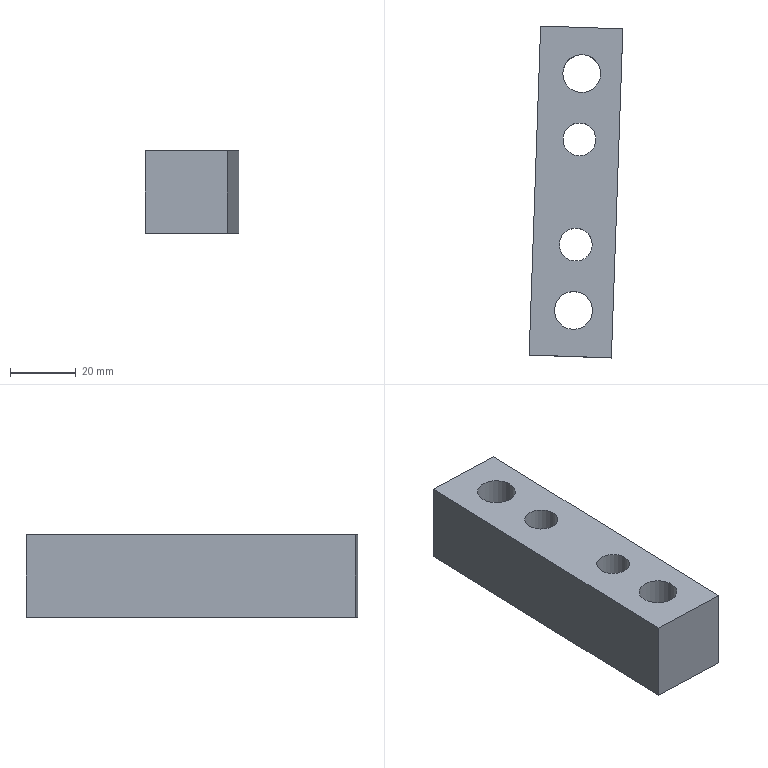Part | NX | features LB-12 2 | 1 solid | 10 faces | box 28.474 x 100.811 x 25 mm | volume 53373 mm3 | plane 6 | cylinder 4 | commonest cylinder face diameters 10 x2 11.507 x2
STEP:
#1=CARTESIAN_POINT('',(3735.733,-918.048,818.716));
#2=VERTEX_POINT('',#1);
#3=CARTESIAN_POINT('',(3732.243,-1017.987,818.716));
#4=VERTEX_POINT('',#3);
#5=CARTESIAN_POINT('',(3734.965,-940.035,818.716));
#6=DIRECTION('',(-0.0349,-0.9994,0.));
#7=VECTOR('',#6,1000.);
#8=LINE('',#5,#7);
#9=EDGE_CURVE('',#2,#4,#8,.T.);
#10=ORIENTED_EDGE('',*,*,#9,.F.);
#11=CARTESIAN_POINT('',(3735.733,-918.048,793.716));
#12=VERTEX_POINT('',#11);
#13=CARTESIAN_POINT('',(3735.733,-918.048,804.216));
#14=DIRECTION('',(0.000000002,0.,-1.));
#15=VECTOR('',#14,1000.);
#16=LINE('',#13,#15);
#17=EDGE_CURVE('',#12,#2,#16,.F.);
#18=ORIENTED_EDGE('',*,*,#17,.F.);
#19=CARTESIAN_POINT('',(3732.243,-1017.987,793.716));
#20=VERTEX_POINT('',#19);
#21=CARTESIAN_POINT('',(3762.984,-137.577,793.716));
#22=DIRECTION('',(0.0349,0.9994,0.));
#23=VECTOR('',#22,1000.);
#24=LINE('',#21,#23);
#25=EDGE_CURVE('',#12,#20,#24,.F.);
#26=ORIENTED_EDGE('',*,*,#25,.T.);
#27=CARTESIAN_POINT('',(3732.243,-1017.987,840.896));
#28=DIRECTION('',(-0.000000002,0.,1.));
#29=VECTOR('',#28,1000.);
#30=LINE('',#27,#29);
#31=EDGE_CURVE('',#4,#20,#30,.F.);
#32=ORIENTED_EDGE('',*,*,#31,.F.);
#33=EDGE_LOOP('',(#10,#18,#26,#32));
#34=FACE_BOUND('',#33,.T.);
#35=CARTESIAN_POINT('',(3734.965,-940.035,821.216));
#36=DIRECTION('',(-0.9994,0.0349,-0.000000002));
#37=DIRECTION('',(0.0349,0.9994,0.));
#38=AXIS2_PLACEMENT_3D('',#35,#36,#37);
#39=PLANE('',#38);
#40=ADVANCED_FACE('',(#34),#39,.T.);
#41=CARTESIAN_POINT('',(3757.228,-1018.86,818.716));
#42=VERTEX_POINT('',#41);
#43=CARTESIAN_POINT('',(3757.228,-1018.86,793.716));
#44=VERTEX_POINT('',#43);
#45=CARTESIAN_POINT('',(3757.228,-1018.86,840.896));
#46=DIRECTION('',(-0.000000002,0.,1.));
#47=VECTOR('',#46,1000.);
#48=LINE('',#45,#47);
#49=EDGE_CURVE('',#42,#44,#48,.F.);
#50=ORIENTED_EDGE('',*,*,#49,.T.);
#51=CARTESIAN_POINT('',(3760.717,-918.92,793.716));
#52=VERTEX_POINT('',#51);
#53=CARTESIAN_POINT('',(3787.969,-138.449,793.716));
#54=DIRECTION('',(0.0349,0.9994,0.));
#55=VECTOR('',#54,1000.);
#56=LINE('',#53,#55);
#57=EDGE_CURVE('',#52,#44,#56,.F.);
#58=ORIENTED_EDGE('',*,*,#57,.F.);
#59=CARTESIAN_POINT('',(3760.717,-918.92,818.716));
#60=VERTEX_POINT('',#59);
#61=CARTESIAN_POINT('',(3760.717,-918.92,804.216));
#62=DIRECTION('',(-0.000000002,0.,1.));
#63=VECTOR('',#62,1000.);
#64=LINE('',#61,#63);
#65=EDGE_CURVE('',#52,#60,#64,.T.);
#66=ORIENTED_EDGE('',*,*,#65,.T.);
#67=CARTESIAN_POINT('',(3766.704,-747.45,818.716));
#68=DIRECTION('',(0.0349,0.9994,0.));
#69=VECTOR('',#68,1000.);
#70=LINE('',#67,#69);
#71=EDGE_CURVE('',#42,#60,#70,.T.);
#72=ORIENTED_EDGE('',*,*,#71,.F.);
#73=EDGE_LOOP('',(#50,#58,#66,#72));
#74=FACE_BOUND('',#73,.T.);
#75=CARTESIAN_POINT('',(3759.95,-940.907,821.216));
#76=DIRECTION('',(-0.9994,0.0349,-0.000000002));
#77=DIRECTION('',(0.0349,0.9994,0.));
#78=AXIS2_PLACEMENT_3D('',#75,#76,#77);
#79=PLANE('',#78);
#80=ADVANCED_FACE('',(#74),#79,.F.);
#81=ORIENTED_EDGE('',*,*,#49,.F.);
#82=CARTESIAN_POINT('',(3757.228,-1018.86,818.716));
#83=DIRECTION('',(0.9994,-0.0349,0.000000002));
#84=VECTOR('',#83,1000.);
#85=LINE('',#82,#84);
#86=EDGE_CURVE('',#42,#4,#85,.F.);
#87=ORIENTED_EDGE('',*,*,#86,.T.);
#88=ORIENTED_EDGE('',*,*,#31,.T.);
#89=CARTESIAN_POINT('',(3757.228,-1018.86,793.716));
#90=DIRECTION('',(0.9994,-0.0349,0.000000004));
#91=VECTOR('',#90,1000.);
#92=LINE('',#89,#91);
#93=EDGE_CURVE('',#20,#44,#92,.T.);
#94=ORIENTED_EDGE('',*,*,#93,.T.);
#95=EDGE_LOOP('',(#81,#87,#88,#94));
#96=FACE_BOUND('',#95,.T.);
#97=CARTESIAN_POINT('',(3757.228,-1018.86,840.896));
#98=DIRECTION('',(-0.0349,-0.9994,0.));
#99=DIRECTION('',(0.000000002,0.,-1.));
#100=AXIS2_PLACEMENT_3D('',#97,#98,#99);
#101=PLANE('',#100);
#102=ADVANCED_FACE('',(#96),#101,.T.);
#103=ORIENTED_EDGE('',*,*,#17,.T.);
#104=CARTESIAN_POINT('',(3760.717,-918.92,818.716));
#105=DIRECTION('',(-0.9994,0.0349,-0.000000002));
#106=VECTOR('',#105,1000.);
#107=LINE('',#104,#106);
#108=EDGE_CURVE('',#2,#60,#107,.F.);
#109=ORIENTED_EDGE('',*,*,#108,.T.);
#110=ORIENTED_EDGE('',*,*,#65,.F.);
#111=CARTESIAN_POINT('',(7637.848,-1054.297,793.716));
#112=DIRECTION('',(0.9994,-0.0349,0.000000004));
#113=VECTOR('',#112,1000.);
#114=LINE('',#111,#113);
#115=EDGE_CURVE('',#12,#52,#114,.T.);
#116=ORIENTED_EDGE('',*,*,#115,.F.);
#117=EDGE_LOOP('',(#103,#109,#110,#116));
#118=FACE_BOUND('',#117,.T.);
#119=CARTESIAN_POINT('',(3760.717,-918.92,804.216));
#120=DIRECTION('',(0.0349,0.9994,0.));
#121=DIRECTION('',(-0.000000002,0.,1.));
#122=AXIS2_PLACEMENT_3D('',#119,#120,#121);
#123=PLANE('',#122);
#124=ADVANCED_FACE('',(#118),#123,.T.);
#125=CARTESIAN_POINT('',(3742.538,-952.481,793.716));
#126=VERTEX_POINT('',#125);
#127=CARTESIAN_POINT('',(3747.538,-952.481,793.716));
#128=DIRECTION('',(0.000000004,0.,-1.));
#129=DIRECTION('',(-1.,0.,-0.000000004));
#130=AXIS2_PLACEMENT_3D('',#127,#128,#129);
#131=CIRCLE('',#130,5.);
#132=EDGE_CURVE('',#126,#126,#131,.F.);
#133=ORIENTED_EDGE('',*,*,#132,.T.);
#134=EDGE_LOOP('',(#133));
#135=FACE_BOUND('',#134,.T.);
#136=CARTESIAN_POINT('',(3741.421,-984.461,793.716));
#137=VERTEX_POINT('',#136);
#138=CARTESIAN_POINT('',(3746.421,-984.461,793.716));
#139=DIRECTION('',(0.000000004,0.,-1.));
#140=DIRECTION('',(-1.,0.,-0.000000004));
#141=AXIS2_PLACEMENT_3D('',#138,#139,#140);
#142=CIRCLE('',#141,5.);
#143=EDGE_CURVE('',#137,#137,#142,.F.);
#144=ORIENTED_EDGE('',*,*,#143,.T.);
#145=EDGE_LOOP('',(#144));
#146=FACE_BOUND('',#145,.T.);
#147=CARTESIAN_POINT('',(3742.483,-932.493,793.716));
#148=VERTEX_POINT('',#147);
#149=CARTESIAN_POINT('',(3748.236,-932.493,793.716));
#150=DIRECTION('',(0.000000004,0.,-1.));
#151=DIRECTION('',(-1.,0.,-0.000000004));
#152=AXIS2_PLACEMENT_3D('',#149,#150,#151);
#153=CIRCLE('',#152,5.753);
#154=EDGE_CURVE('',#148,#148,#153,.F.);
#155=ORIENTED_EDGE('',*,*,#154,.T.);
#156=EDGE_LOOP('',(#155));
#157=FACE_BOUND('',#156,.T.);
#158=CARTESIAN_POINT('',(3739.97,-1004.449,793.716));
#159=VERTEX_POINT('',#158);
#160=CARTESIAN_POINT('',(3745.724,-1004.449,793.716));
#161=DIRECTION('',(0.000000004,0.,-1.));
#162=DIRECTION('',(-1.,0.,-0.000000004));
#163=AXIS2_PLACEMENT_3D('',#160,#161,#162);
#164=CIRCLE('',#163,5.753);
#165=EDGE_CURVE('',#159,#159,#164,.F.);
#166=ORIENTED_EDGE('',*,*,#165,.T.);
#167=EDGE_LOOP('',(#166));
#168=FACE_BOUND('',#167,.T.);
#169=ORIENTED_EDGE('',*,*,#25,.F.);
#170=ORIENTED_EDGE('',*,*,#115,.T.);
#171=ORIENTED_EDGE('',*,*,#57,.T.);
#172=ORIENTED_EDGE('',*,*,#93,.F.);
#173=EDGE_LOOP('',(#169,#170,#171,#172));
#174=FACE_BOUND('',#173,.T.);
#175=CARTESIAN_POINT('',(7665.099,-273.826,793.716));
#176=DIRECTION('',(0.000000004,0.,-1.));
#177=DIRECTION('',(0.9976,-0.06975,0.000000004));
#178=AXIS2_PLACEMENT_3D('',#175,#176,#177);
#179=PLANE('',#178);
#180=ADVANCED_FACE('',(#135,#146,#157,#168,#174),#179,.T.);
#181=CARTESIAN_POINT('',(3742.538,-952.481,818.716));
#182=VERTEX_POINT('',#181);
#183=CARTESIAN_POINT('',(3747.538,-952.481,818.716));
#184=DIRECTION('',(0.000000002,0.,-1.));
#185=DIRECTION('',(-1.,0.,-0.000000002));
#186=AXIS2_PLACEMENT_3D('',#183,#184,#185);
#187=CIRCLE('',#186,5.);
#188=EDGE_CURVE('',#182,#182,#187,.T.);
#189=ORIENTED_EDGE('',*,*,#188,.T.);
#190=EDGE_LOOP('',(#189));
#191=FACE_BOUND('',#190,.T.);
#192=CARTESIAN_POINT('',(3741.421,-984.461,818.716));
#193=VERTEX_POINT('',#192);
#194=CARTESIAN_POINT('',(3746.421,-984.461,818.716));
#195=DIRECTION('',(0.000000002,0.,-1.));
#196=DIRECTION('',(-1.,0.,-0.000000002));
#197=AXIS2_PLACEMENT_3D('',#194,#195,#196);
#198=CIRCLE('',#197,5.);
#199=EDGE_CURVE('',#193,#193,#198,.T.);
#200=ORIENTED_EDGE('',*,*,#199,.T.);
#201=EDGE_LOOP('',(#200));
#202=FACE_BOUND('',#201,.T.);
#203=CARTESIAN_POINT('',(3742.483,-932.493,818.716));
#204=VERTEX_POINT('',#203);
#205=CARTESIAN_POINT('',(3748.236,-932.493,818.716));
#206=DIRECTION('',(0.000000002,0.,-1.));
#207=DIRECTION('',(-1.,0.,-0.000000002));
#208=AXIS2_PLACEMENT_3D('',#205,#206,#207);
#209=CIRCLE('',#208,5.753);
#210=EDGE_CURVE('',#204,#204,#209,.T.);
#211=ORIENTED_EDGE('',*,*,#210,.T.);
#212=EDGE_LOOP('',(#211));
#213=FACE_BOUND('',#212,.T.);
#214=CARTESIAN_POINT('',(3739.97,-1004.449,818.716));
#215=VERTEX_POINT('',#214);
#216=CARTESIAN_POINT('',(3745.724,-1004.449,818.716));
#217=DIRECTION('',(0.000000002,0.,-1.));
#218=DIRECTION('',(-1.,0.,-0.000000002));
#219=AXIS2_PLACEMENT_3D('',#216,#217,#218);
#220=CIRCLE('',#219,5.753);
#221=EDGE_CURVE('',#215,#215,#220,.T.);
#222=ORIENTED_EDGE('',*,*,#221,.T.);
#223=EDGE_LOOP('',(#222));
#224=FACE_BOUND('',#223,.T.);
#225=ORIENTED_EDGE('',*,*,#71,.T.);
#226=ORIENTED_EDGE('',*,*,#108,.F.);
#227=ORIENTED_EDGE('',*,*,#9,.T.);
#228=ORIENTED_EDGE('',*,*,#86,.F.);
#229=EDGE_LOOP('',(#225,#226,#227,#228));
#230=FACE_BOUND('',#229,.T.);
#231=CARTESIAN_POINT('',(3761.471,-747.267,818.716));
#232=DIRECTION('',(0.000000002,0.,-1.));
#233=DIRECTION('',(-1.,0.,-0.000000002));
#234=AXIS2_PLACEMENT_3D('',#231,#232,#233);
#235=PLANE('',#234);
#236=ADVANCED_FACE('',(#191,#202,#213,#224,#230),#235,.F.);
#237=ORIENTED_EDGE('',*,*,#221,.F.);
#238=EDGE_LOOP('',(#237));
#239=FACE_BOUND('',#238,.T.);
#240=ORIENTED_EDGE('',*,*,#165,.F.);
#241=EDGE_LOOP('',(#240));
#242=FACE_BOUND('',#241,.T.);
#243=CARTESIAN_POINT('',(3745.724,-1004.449,818.716));
#244=DIRECTION('',(0.,0.,-1.));
#245=DIRECTION('',(1.,0.,0.));
#246=AXIS2_PLACEMENT_3D('',#243,#244,#245);
#247=CYLINDRICAL_SURFACE('',#246,5.753);
#248=ADVANCED_FACE('',(#239,#242),#247,.F.);
#249=ORIENTED_EDGE('',*,*,#210,.F.);
#250=EDGE_LOOP('',(#249));
#251=FACE_BOUND('',#250,.T.);
#252=ORIENTED_EDGE('',*,*,#154,.F.);
#253=EDGE_LOOP('',(#252));
#254=FACE_BOUND('',#253,.T.);
#255=CARTESIAN_POINT('',(3748.236,-932.493,818.716));
#256=DIRECTION('',(0.,0.,-1.));
#257=DIRECTION('',(1.,0.,0.));
#258=AXIS2_PLACEMENT_3D('',#255,#256,#257);
#259=CYLINDRICAL_SURFACE('',#258,5.753);
#260=ADVANCED_FACE('',(#251,#254),#259,.F.);
#261=ORIENTED_EDGE('',*,*,#199,.F.);
#262=EDGE_LOOP('',(#261));
#263=FACE_BOUND('',#262,.T.);
#264=ORIENTED_EDGE('',*,*,#143,.F.);
#265=EDGE_LOOP('',(#264));
#266=FACE_BOUND('',#265,.T.);
#267=CARTESIAN_POINT('',(3746.421,-984.461,818.716));
#268=DIRECTION('',(0.,0.,-1.));
#269=DIRECTION('',(1.,0.,0.));
#270=AXIS2_PLACEMENT_3D('',#267,#268,#269);
#271=CYLINDRICAL_SURFACE('',#270,5.);
#272=ADVANCED_FACE('',(#263,#266),#271,.F.);
#273=ORIENTED_EDGE('',*,*,#188,.F.);
#274=EDGE_LOOP('',(#273));
#275=FACE_BOUND('',#274,.T.);
#276=ORIENTED_EDGE('',*,*,#132,.F.);
#277=EDGE_LOOP('',(#276));
#278=FACE_BOUND('',#277,.T.);
#279=CARTESIAN_POINT('',(3747.538,-952.481,818.716));
#280=DIRECTION('',(0.,0.,-1.));
#281=DIRECTION('',(1.,0.,0.));
#282=AXIS2_PLACEMENT_3D('',#279,#280,#281);
#283=CYLINDRICAL_SURFACE('',#282,5.);
#284=ADVANCED_FACE('',(#275,#278),#283,.F.);
#285=CLOSED_SHELL('',(#40,#80,#102,#124,#180,#236,#248,#260,#272,#284));
#286=MANIFOLD_SOLID_BREP('',#285);
#287=(LENGTH_UNIT()NAMED_UNIT(*)SI_UNIT(.MILLI.,.METRE.));
#288=UNCERTAINTY_MEASURE_WITH_UNIT(LENGTH_MEASURE(0.00001),#287,'','');
#289=(NAMED_UNIT(*)PLANE_ANGLE_UNIT()SI_UNIT($,.RADIAN.));
#290=(NAMED_UNIT(*)SI_UNIT($,.STERADIAN.)SOLID_ANGLE_UNIT());
#291=(GEOMETRIC_REPRESENTATION_CONTEXT(3)GLOBAL_UNCERTAINTY_ASSIGNED_CONTEXT((#288))GLOBAL_UNIT_ASSIGNED_CONTEXT((#287,#289,#290))REPRESENTATION_CONTEXT('',''));
#292=ADVANCED_BREP_SHAPE_REPRESENTATION('',(#286),#291);